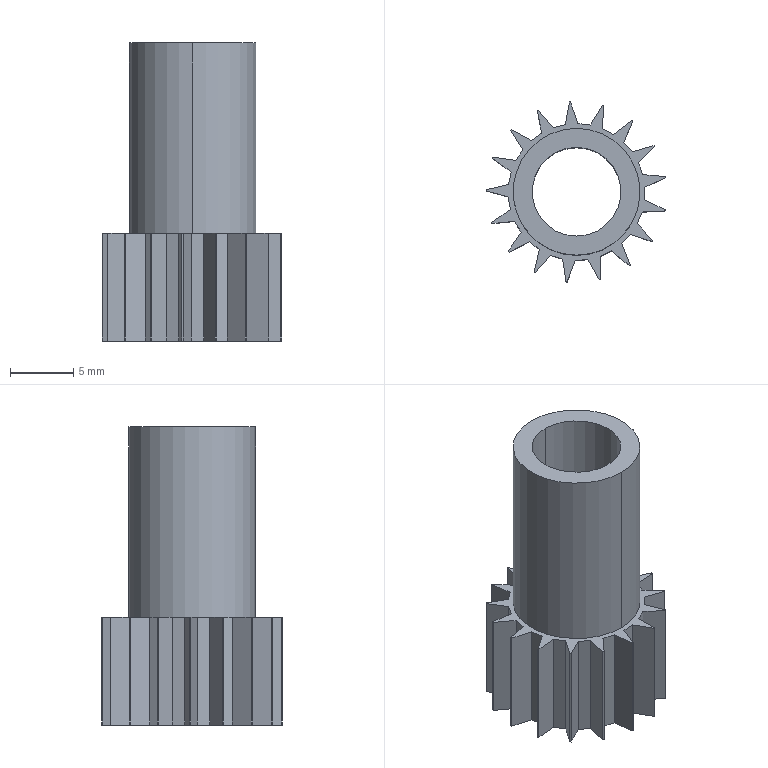Part | STEP file | 2026.6.15-Main Assembly图.sldasm-Part-120 | 1 solid | 75 faces | box 14.16 x 14.195 x 23.5 mm | volume 1185 mm3 | plane 54 | cylinder 21 | commonest cylinder face diameters 14.25 x17 7 x2 10 x2